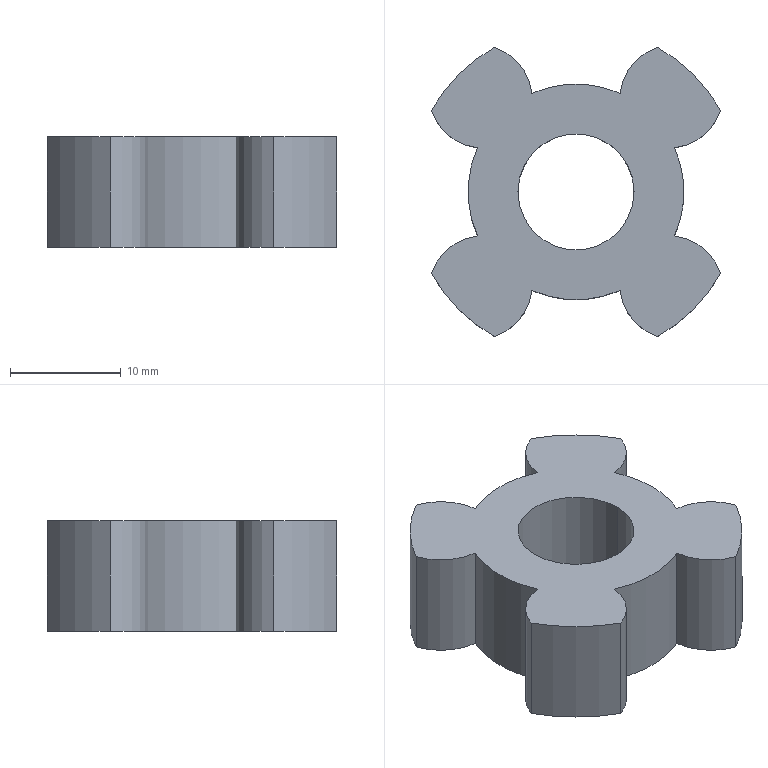Part | SolidWorks | features BaseBody 1 | 1 solid | 21 faces | box 26.134 x 26.134 x 10 mm | volume 3952 mm3 | cylinder 19 | plane 2 | commonest cylinder face diameters 10 x8 19.5 x5 30 x4 10.5 x2
STEP:
#1=CARTESIAN_POINT('',(5.25,0.,-5.));
#2=VERTEX_POINT('',#1);
#3=CARTESIAN_POINT('',(-5.25,0.,-5.));
#4=VERTEX_POINT('',#3);
#5=CARTESIAN_POINT('',(0.,0.,-5.));
#6=DIRECTION('',(0.,0.,-1.));
#7=DIRECTION('',(1.,0.,0.));
#8=AXIS2_PLACEMENT_3D('',#5,#6,#7);
#9=CIRCLE('',#8,5.25);
#10=EDGE_CURVE('',#2,#4,#9,.T.);
#11=ORIENTED_EDGE('',*,*,#10,.T.);
#12=CARTESIAN_POINT('',(-5.25,0.,5.));
#13=VERTEX_POINT('',#12);
#14=CARTESIAN_POINT('',(-5.25,0.,-5.));
#15=DIRECTION('',(0.,0.,1.));
#16=VECTOR('',#15,1000.);
#17=LINE('',#14,#16);
#18=EDGE_CURVE('',#4,#13,#17,.T.);
#19=ORIENTED_EDGE('',*,*,#18,.T.);
#20=CARTESIAN_POINT('',(5.25,0.,5.));
#21=VERTEX_POINT('',#20);
#22=CARTESIAN_POINT('',(0.,0.,5.));
#23=DIRECTION('',(0.,0.,-1.));
#24=DIRECTION('',(1.,0.,0.));
#25=AXIS2_PLACEMENT_3D('',#22,#23,#24);
#26=CIRCLE('',#25,5.25);
#27=EDGE_CURVE('',#21,#13,#26,.T.);
#28=ORIENTED_EDGE('',*,*,#27,.F.);
#29=CARTESIAN_POINT('',(5.25,0.,-5.));
#30=DIRECTION('',(0.,0.,1.));
#31=VECTOR('',#30,1000.);
#32=LINE('',#29,#31);
#33=EDGE_CURVE('',#2,#21,#32,.T.);
#34=ORIENTED_EDGE('',*,*,#33,.F.);
#35=EDGE_LOOP('',(#11,#19,#28,#34));
#36=FACE_OUTER_BOUND('',#35,.T.);
#37=CARTESIAN_POINT('',(0.,0.,-5.));
#38=DIRECTION('',(0.,0.,1.));
#39=DIRECTION('',(1.,0.,0.));
#40=AXIS2_PLACEMENT_3D('',#37,#38,#39);
#41=CYLINDRICAL_SURFACE('',#40,5.25);
#42=ADVANCED_FACE('',(#36),#41,.F.);
#43=CARTESIAN_POINT('',(8.901,-3.98,-5.));
#44=VERTEX_POINT('',#43);
#45=CARTESIAN_POINT('',(9.75,0.,-5.));
#46=VERTEX_POINT('',#45);
#47=CARTESIAN_POINT('',(0.,0.,-5.));
#48=DIRECTION('',(0.,0.,1.));
#49=DIRECTION('',(1.,0.,0.));
#50=AXIS2_PLACEMENT_3D('',#47,#48,#49);
#51=CIRCLE('',#50,9.75);
#52=EDGE_CURVE('',#44,#46,#51,.T.);
#53=ORIENTED_EDGE('',*,*,#52,.T.);
#54=CARTESIAN_POINT('',(9.75,0.,5.));
#55=VERTEX_POINT('',#54);
#56=CARTESIAN_POINT('',(9.75,0.,0.));
#57=DIRECTION('',(0.,0.,1.));
#58=VECTOR('',#57,1000.);
#59=LINE('',#56,#58);
#60=EDGE_CURVE('',#46,#55,#59,.T.);
#61=ORIENTED_EDGE('',*,*,#60,.T.);
#62=CARTESIAN_POINT('',(8.901,-3.98,5.));
#63=VERTEX_POINT('',#62);
#64=CARTESIAN_POINT('',(0.,0.,5.));
#65=DIRECTION('',(0.,0.,-1.));
#66=DIRECTION('',(1.,0.,0.));
#67=AXIS2_PLACEMENT_3D('',#64,#65,#66);
#68=CIRCLE('',#67,9.75);
#69=EDGE_CURVE('',#55,#63,#68,.T.);
#70=ORIENTED_EDGE('',*,*,#69,.T.);
#71=CARTESIAN_POINT('',(8.901,-3.98,0.));
#72=DIRECTION('',(0.,0.,-1.));
#73=VECTOR('',#72,1000.);
#74=LINE('',#71,#73);
#75=EDGE_CURVE('',#63,#44,#74,.T.);
#76=ORIENTED_EDGE('',*,*,#75,.T.);
#77=EDGE_LOOP('',(#53,#61,#70,#76));
#78=FACE_OUTER_BOUND('',#77,.T.);
#79=CARTESIAN_POINT('',(0.,0.,0.));
#80=DIRECTION('',(0.,0.,1.));
#81=DIRECTION('',(1.,0.,0.));
#82=AXIS2_PLACEMENT_3D('',#79,#80,#81);
#83=CYLINDRICAL_SURFACE('',#82,9.75);
#84=ADVANCED_FACE('',(#78),#83,.T.);
#85=ORIENTED_EDGE('',*,*,#10,.F.);
#86=CARTESIAN_POINT('',(0.,0.,-5.));
#87=DIRECTION('',(0.,0.,-1.));
#88=DIRECTION('',(1.,0.,0.));
#89=AXIS2_PLACEMENT_3D('',#86,#87,#88);
#90=CIRCLE('',#89,5.25);
#91=EDGE_CURVE('',#4,#2,#90,.T.);
#92=ORIENTED_EDGE('',*,*,#91,.F.);
#93=EDGE_LOOP('',(#85,#92));
#94=FACE_BOUND('',#93,.T.);
#95=CARTESIAN_POINT('',(7.366,13.067,-5.));
#96=VERTEX_POINT('',#95);
#97=CARTESIAN_POINT('',(3.98,8.901,-5.));
#98=VERTEX_POINT('',#97);
#99=CARTESIAN_POINT('',(8.946,8.323,-5.));
#100=DIRECTION('',(0.,0.,1.));
#101=DIRECTION('',(1.,0.,0.));
#102=AXIS2_PLACEMENT_3D('',#99,#100,#101);
#103=CIRCLE('',#102,5.);
#104=EDGE_CURVE('',#96,#98,#103,.T.);
#105=ORIENTED_EDGE('',*,*,#104,.F.);
#106=CARTESIAN_POINT('',(13.067,7.366,-5.));
#107=VERTEX_POINT('',#106);
#108=CARTESIAN_POINT('',(0.,0.,-5.));
#109=DIRECTION('',(0.,0.,1.));
#110=DIRECTION('',(1.,0.,0.));
#111=AXIS2_PLACEMENT_3D('',#108,#109,#110);
#112=CIRCLE('',#111,15.);
#113=EDGE_CURVE('',#107,#96,#112,.T.);
#114=ORIENTED_EDGE('',*,*,#113,.F.);
#115=CARTESIAN_POINT('',(8.901,3.98,-5.));
#116=VERTEX_POINT('',#115);
#117=CARTESIAN_POINT('',(8.323,8.946,-5.));
#118=DIRECTION('',(0.,0.,1.));
#119=DIRECTION('',(1.,0.,0.));
#120=AXIS2_PLACEMENT_3D('',#117,#118,#119);
#121=CIRCLE('',#120,5.);
#122=EDGE_CURVE('',#116,#107,#121,.T.);
#123=ORIENTED_EDGE('',*,*,#122,.F.);
#124=CARTESIAN_POINT('',(0.,0.,-5.));
#125=DIRECTION('',(0.,0.,1.));
#126=DIRECTION('',(1.,0.,0.));
#127=AXIS2_PLACEMENT_3D('',#124,#125,#126);
#128=CIRCLE('',#127,9.75);
#129=EDGE_CURVE('',#46,#116,#128,.T.);
#130=ORIENTED_EDGE('',*,*,#129,.F.);
#131=ORIENTED_EDGE('',*,*,#52,.F.);
#132=CARTESIAN_POINT('',(13.067,-7.366,-5.));
#133=VERTEX_POINT('',#132);
#134=CARTESIAN_POINT('',(8.323,-8.946,-5.));
#135=DIRECTION('',(0.,0.,1.));
#136=DIRECTION('',(1.,0.,0.));
#137=AXIS2_PLACEMENT_3D('',#134,#135,#136);
#138=CIRCLE('',#137,5.);
#139=EDGE_CURVE('',#133,#44,#138,.T.);
#140=ORIENTED_EDGE('',*,*,#139,.F.);
#141=CARTESIAN_POINT('',(7.366,-13.067,-5.));
#142=VERTEX_POINT('',#141);
#143=CARTESIAN_POINT('',(0.,0.,-5.));
#144=DIRECTION('',(0.,0.,1.));
#145=DIRECTION('',(1.,0.,0.));
#146=AXIS2_PLACEMENT_3D('',#143,#144,#145);
#147=CIRCLE('',#146,15.);
#148=EDGE_CURVE('',#142,#133,#147,.T.);
#149=ORIENTED_EDGE('',*,*,#148,.F.);
#150=CARTESIAN_POINT('',(3.98,-8.901,-5.));
#151=VERTEX_POINT('',#150);
#152=CARTESIAN_POINT('',(8.946,-8.323,-5.));
#153=DIRECTION('',(0.,0.,1.));
#154=DIRECTION('',(1.,0.,0.));
#155=AXIS2_PLACEMENT_3D('',#152,#153,#154);
#156=CIRCLE('',#155,5.);
#157=EDGE_CURVE('',#151,#142,#156,.T.);
#158=ORIENTED_EDGE('',*,*,#157,.F.);
#159=CARTESIAN_POINT('',(-3.98,-8.901,-5.));
#160=VERTEX_POINT('',#159);
#161=CARTESIAN_POINT('',(0.,0.,-5.));
#162=DIRECTION('',(0.,0.,1.));
#163=DIRECTION('',(1.,0.,0.));
#164=AXIS2_PLACEMENT_3D('',#161,#162,#163);
#165=CIRCLE('',#164,9.75);
#166=EDGE_CURVE('',#160,#151,#165,.T.);
#167=ORIENTED_EDGE('',*,*,#166,.F.);
#168=CARTESIAN_POINT('',(-7.366,-13.067,-5.));
#169=VERTEX_POINT('',#168);
#170=CARTESIAN_POINT('',(-8.946,-8.323,-5.));
#171=DIRECTION('',(0.,0.,1.));
#172=DIRECTION('',(1.,0.,0.));
#173=AXIS2_PLACEMENT_3D('',#170,#171,#172);
#174=CIRCLE('',#173,5.);
#175=EDGE_CURVE('',#169,#160,#174,.T.);
#176=ORIENTED_EDGE('',*,*,#175,.F.);
#177=CARTESIAN_POINT('',(-13.067,-7.366,-5.));
#178=VERTEX_POINT('',#177);
#179=CARTESIAN_POINT('',(0.,0.,-5.));
#180=DIRECTION('',(0.,0.,1.));
#181=DIRECTION('',(1.,0.,0.));
#182=AXIS2_PLACEMENT_3D('',#179,#180,#181);
#183=CIRCLE('',#182,15.);
#184=EDGE_CURVE('',#178,#169,#183,.T.);
#185=ORIENTED_EDGE('',*,*,#184,.F.);
#186=CARTESIAN_POINT('',(-8.901,-3.98,-5.));
#187=VERTEX_POINT('',#186);
#188=CARTESIAN_POINT('',(-8.323,-8.946,-5.));
#189=DIRECTION('',(0.,0.,1.));
#190=DIRECTION('',(1.,0.,0.));
#191=AXIS2_PLACEMENT_3D('',#188,#189,#190);
#192=CIRCLE('',#191,5.);
#193=EDGE_CURVE('',#187,#178,#192,.T.);
#194=ORIENTED_EDGE('',*,*,#193,.F.);
#195=CARTESIAN_POINT('',(-8.901,3.98,-5.));
#196=VERTEX_POINT('',#195);
#197=CARTESIAN_POINT('',(0.,0.,-5.));
#198=DIRECTION('',(0.,0.,1.));
#199=DIRECTION('',(1.,0.,0.));
#200=AXIS2_PLACEMENT_3D('',#197,#198,#199);
#201=CIRCLE('',#200,9.75);
#202=EDGE_CURVE('',#196,#187,#201,.T.);
#203=ORIENTED_EDGE('',*,*,#202,.F.);
#204=CARTESIAN_POINT('',(-13.067,7.366,-5.));
#205=VERTEX_POINT('',#204);
#206=CARTESIAN_POINT('',(-8.323,8.946,-5.));
#207=DIRECTION('',(0.,0.,1.));
#208=DIRECTION('',(1.,0.,0.));
#209=AXIS2_PLACEMENT_3D('',#206,#207,#208);
#210=CIRCLE('',#209,5.);
#211=EDGE_CURVE('',#205,#196,#210,.T.);
#212=ORIENTED_EDGE('',*,*,#211,.F.);
#213=CARTESIAN_POINT('',(-7.366,13.067,-5.));
#214=VERTEX_POINT('',#213);
#215=CARTESIAN_POINT('',(0.,0.,-5.));
#216=DIRECTION('',(0.,0.,1.));
#217=DIRECTION('',(1.,0.,0.));
#218=AXIS2_PLACEMENT_3D('',#215,#216,#217);
#219=CIRCLE('',#218,15.);
#220=EDGE_CURVE('',#214,#205,#219,.T.);
#221=ORIENTED_EDGE('',*,*,#220,.F.);
#222=CARTESIAN_POINT('',(-3.98,8.901,-5.));
#223=VERTEX_POINT('',#222);
#224=CARTESIAN_POINT('',(-8.946,8.323,-5.));
#225=DIRECTION('',(0.,0.,1.));
#226=DIRECTION('',(1.,0.,0.));
#227=AXIS2_PLACEMENT_3D('',#224,#225,#226);
#228=CIRCLE('',#227,5.);
#229=EDGE_CURVE('',#223,#214,#228,.T.);
#230=ORIENTED_EDGE('',*,*,#229,.F.);
#231=CARTESIAN_POINT('',(0.,0.,-5.));
#232=DIRECTION('',(0.,0.,1.));
#233=DIRECTION('',(1.,0.,0.));
#234=AXIS2_PLACEMENT_3D('',#231,#232,#233);
#235=CIRCLE('',#234,9.75);
#236=EDGE_CURVE('',#98,#223,#235,.T.);
#237=ORIENTED_EDGE('',*,*,#236,.F.);
#238=EDGE_LOOP('',(#105,#114,#123,#130,#131,#140,#149,#158,#167,#176,#185,#194,#203,#212,#221,#230,#237));
#239=FACE_OUTER_BOUND('',#238,.T.);
#240=CARTESIAN_POINT('',(0.,0.,-5.));
#241=DIRECTION('',(0.,0.,1.));
#242=DIRECTION('',(1.,0.,0.));
#243=AXIS2_PLACEMENT_3D('',#240,#241,#242);
#244=PLANE('',#243);
#245=ADVANCED_FACE('',(#94,#239),#244,.F.);
#246=ORIENTED_EDGE('',*,*,#18,.F.);
#247=ORIENTED_EDGE('',*,*,#91,.T.);
#248=ORIENTED_EDGE('',*,*,#33,.T.);
#249=CARTESIAN_POINT('',(0.,0.,5.));
#250=DIRECTION('',(0.,0.,-1.));
#251=DIRECTION('',(1.,0.,0.));
#252=AXIS2_PLACEMENT_3D('',#249,#250,#251);
#253=CIRCLE('',#252,5.25);
#254=EDGE_CURVE('',#13,#21,#253,.T.);
#255=ORIENTED_EDGE('',*,*,#254,.F.);
#256=EDGE_LOOP('',(#246,#247,#248,#255));
#257=FACE_OUTER_BOUND('',#256,.T.);
#258=CARTESIAN_POINT('',(0.,0.,-5.));
#259=DIRECTION('',(0.,0.,1.));
#260=DIRECTION('',(1.,0.,0.));
#261=AXIS2_PLACEMENT_3D('',#258,#259,#260);
#262=CYLINDRICAL_SURFACE('',#261,5.25);
#263=ADVANCED_FACE('',(#257),#262,.F.);
#264=CARTESIAN_POINT('',(-3.98,8.901,5.));
#265=VERTEX_POINT('',#264);
#266=CARTESIAN_POINT('',(3.98,8.901,5.));
#267=VERTEX_POINT('',#266);
#268=CARTESIAN_POINT('',(0.,0.,5.));
#269=DIRECTION('',(0.,0.,-1.));
#270=DIRECTION('',(1.,0.,0.));
#271=AXIS2_PLACEMENT_3D('',#268,#269,#270);
#272=CIRCLE('',#271,9.75);
#273=EDGE_CURVE('',#265,#267,#272,.T.);
#274=ORIENTED_EDGE('',*,*,#273,.T.);
#275=CARTESIAN_POINT('',(3.98,8.901,0.));
#276=DIRECTION('',(0.,0.,-1.));
#277=VECTOR('',#276,1000.);
#278=LINE('',#275,#277);
#279=EDGE_CURVE('',#267,#98,#278,.T.);
#280=ORIENTED_EDGE('',*,*,#279,.T.);
#281=ORIENTED_EDGE('',*,*,#236,.T.);
#282=CARTESIAN_POINT('',(-3.98,8.901,0.));
#283=DIRECTION('',(0.,0.,1.));
#284=VECTOR('',#283,1000.);
#285=LINE('',#282,#284);
#286=EDGE_CURVE('',#223,#265,#285,.T.);
#287=ORIENTED_EDGE('',*,*,#286,.T.);
#288=EDGE_LOOP('',(#274,#280,#281,#287));
#289=FACE_OUTER_BOUND('',#288,.T.);
#290=CARTESIAN_POINT('',(0.,0.,0.));
#291=DIRECTION('',(0.,0.,1.));
#292=DIRECTION('',(1.,0.,0.));
#293=AXIS2_PLACEMENT_3D('',#290,#291,#292);
#294=CYLINDRICAL_SURFACE('',#293,9.75);
#295=ADVANCED_FACE('',(#289),#294,.T.);
#296=CARTESIAN_POINT('',(7.366,13.067,5.));
#297=VERTEX_POINT('',#296);
#298=CARTESIAN_POINT('',(8.946,8.323,5.));
#299=DIRECTION('',(0.,0.,-1.));
#300=DIRECTION('',(1.,0.,0.));
#301=AXIS2_PLACEMENT_3D('',#298,#299,#300);
#302=CIRCLE('',#301,5.);
#303=EDGE_CURVE('',#267,#297,#302,.T.);
#304=ORIENTED_EDGE('',*,*,#303,.T.);
#305=CARTESIAN_POINT('',(7.366,13.067,0.));
#306=DIRECTION('',(0.,0.,-1.));
#307=VECTOR('',#306,1000.);
#308=LINE('',#305,#307);
#309=EDGE_CURVE('',#297,#96,#308,.T.);
#310=ORIENTED_EDGE('',*,*,#309,.T.);
#311=ORIENTED_EDGE('',*,*,#104,.T.);
#312=ORIENTED_EDGE('',*,*,#279,.F.);
#313=EDGE_LOOP('',(#304,#310,#311,#312));
#314=FACE_OUTER_BOUND('',#313,.T.);
#315=CARTESIAN_POINT('',(8.946,8.323,0.));
#316=DIRECTION('',(0.,0.,1.));
#317=DIRECTION('',(1.,0.,0.));
#318=AXIS2_PLACEMENT_3D('',#315,#316,#317);
#319=CYLINDRICAL_SURFACE('',#318,5.);
#320=ADVANCED_FACE('',(#314),#319,.T.);
#321=CARTESIAN_POINT('',(13.067,7.366,5.));
#322=VERTEX_POINT('',#321);
#323=CARTESIAN_POINT('',(0.,0.,5.));
#324=DIRECTION('',(0.,0.,-1.));
#325=DIRECTION('',(1.,0.,0.));
#326=AXIS2_PLACEMENT_3D('',#323,#324,#325);
#327=CIRCLE('',#326,15.);
#328=EDGE_CURVE('',#297,#322,#327,.T.);
#329=ORIENTED_EDGE('',*,*,#328,.T.);
#330=CARTESIAN_POINT('',(13.067,7.366,0.));
#331=DIRECTION('',(0.,0.,-1.));
#332=VECTOR('',#331,1000.);
#333=LINE('',#330,#332);
#334=EDGE_CURVE('',#322,#107,#333,.T.);
#335=ORIENTED_EDGE('',*,*,#334,.T.);
#336=ORIENTED_EDGE('',*,*,#113,.T.);
#337=ORIENTED_EDGE('',*,*,#309,.F.);
#338=EDGE_LOOP('',(#329,#335,#336,#337));
#339=FACE_OUTER_BOUND('',#338,.T.);
#340=CARTESIAN_POINT('',(0.,0.,0.));
#341=DIRECTION('',(0.,0.,1.));
#342=DIRECTION('',(1.,0.,0.));
#343=AXIS2_PLACEMENT_3D('',#340,#341,#342);
#344=CYLINDRICAL_SURFACE('',#343,15.);
#345=ADVANCED_FACE('',(#339),#344,.T.);
#346=CARTESIAN_POINT('',(8.901,3.98,5.));
#347=VERTEX_POINT('',#346);
#348=CARTESIAN_POINT('',(8.323,8.946,5.));
#349=DIRECTION('',(0.,0.,-1.));
#350=DIRECTION('',(1.,0.,0.));
#351=AXIS2_PLACEMENT_3D('',#348,#349,#350);
#352=CIRCLE('',#351,5.);
#353=EDGE_CURVE('',#322,#347,#352,.T.);
#354=ORIENTED_EDGE('',*,*,#353,.T.);
#355=CARTESIAN_POINT('',(8.901,3.98,0.));
#356=DIRECTION('',(0.,0.,-1.));
#357=VECTOR('',#356,1000.);
#358=LINE('',#355,#357);
#359=EDGE_CURVE('',#347,#116,#358,.T.);
#360=ORIENTED_EDGE('',*,*,#359,.T.);
#361=ORIENTED_EDGE('',*,*,#122,.T.);
#362=ORIENTED_EDGE('',*,*,#334,.F.);
#363=EDGE_LOOP('',(#354,#360,#361,#362));
#364=FACE_OUTER_BOUND('',#363,.T.);
#365=CARTESIAN_POINT('',(8.323,8.946,0.));
#366=DIRECTION('',(0.,0.,1.));
#367=DIRECTION('',(1.,0.,0.));
#368=AXIS2_PLACEMENT_3D('',#365,#366,#367);
#369=CYLINDRICAL_SURFACE('',#368,5.);
#370=ADVANCED_FACE('',(#364),#369,.T.);
#371=ORIENTED_EDGE('',*,*,#60,.F.);
#372=ORIENTED_EDGE('',*,*,#129,.T.);
#373=ORIENTED_EDGE('',*,*,#359,.F.);
#374=CARTESIAN_POINT('',(0.,0.,5.));
#375=DIRECTION('',(0.,0.,-1.));
#376=DIRECTION('',(1.,0.,0.));
#377=AXIS2_PLACEMENT_3D('',#374,#375,#376);
#378=CIRCLE('',#377,9.75);
#379=EDGE_CURVE('',#347,#55,#378,.T.);
#380=ORIENTED_EDGE('',*,*,#379,.T.);
#381=EDGE_LOOP('',(#371,#372,#373,#380));
#382=FACE_OUTER_BOUND('',#381,.T.);
#383=CARTESIAN_POINT('',(0.,0.,0.));
#384=DIRECTION('',(0.,0.,1.));
#385=DIRECTION('',(1.,0.,0.));
#386=AXIS2_PLACEMENT_3D('',#383,#384,#385);
#387=CYLINDRICAL_SURFACE('',#386,9.75);
#388=ADVANCED_FACE('',(#382),#387,.T.);
#389=CARTESIAN_POINT('',(13.067,-7.366,5.));
#390=VERTEX_POINT('',#389);
#391=CARTESIAN_POINT('',(8.323,-8.946,5.));
#392=DIRECTION('',(0.,0.,-1.));
#393=DIRECTION('',(1.,0.,0.));
#394=AXIS2_PLACEMENT_3D('',#391,#392,#393);
#395=CIRCLE('',#394,5.);
#396=EDGE_CURVE('',#63,#390,#395,.T.);
#397=ORIENTED_EDGE('',*,*,#396,.T.);
#398=CARTESIAN_POINT('',(13.067,-7.366,0.));
#399=DIRECTION('',(0.,0.,-1.));
#400=VECTOR('',#399,1000.);
#401=LINE('',#398,#400);
#402=EDGE_CURVE('',#390,#133,#401,.T.);
#403=ORIENTED_EDGE('',*,*,#402,.T.);
#404=ORIENTED_EDGE('',*,*,#139,.T.);
#405=ORIENTED_EDGE('',*,*,#75,.F.);
#406=EDGE_LOOP('',(#397,#403,#404,#405));
#407=FACE_OUTER_BOUND('',#406,.T.);
#408=CARTESIAN_POINT('',(8.323,-8.946,0.));
#409=DIRECTION('',(0.,0.,1.));
#410=DIRECTION('',(1.,0.,0.));
#411=AXIS2_PLACEMENT_3D('',#408,#409,#410);
#412=CYLINDRICAL_SURFACE('',#411,5.);
#413=ADVANCED_FACE('',(#407),#412,.T.);
#414=CARTESIAN_POINT('',(7.366,-13.067,5.));
#415=VERTEX_POINT('',#414);
#416=CARTESIAN_POINT('',(0.,0.,5.));
#417=DIRECTION('',(0.,0.,-1.));
#418=DIRECTION('',(1.,0.,0.));
#419=AXIS2_PLACEMENT_3D('',#416,#417,#418);
#420=CIRCLE('',#419,15.);
#421=EDGE_CURVE('',#390,#415,#420,.T.);
#422=ORIENTED_EDGE('',*,*,#421,.T.);
#423=CARTESIAN_POINT('',(7.366,-13.067,0.));
#424=DIRECTION('',(0.,0.,-1.));
#425=VECTOR('',#424,1000.);
#426=LINE('',#423,#425);
#427=EDGE_CURVE('',#415,#142,#426,.T.);
#428=ORIENTED_EDGE('',*,*,#427,.T.);
#429=ORIENTED_EDGE('',*,*,#148,.T.);
#430=ORIENTED_EDGE('',*,*,#402,.F.);
#431=EDGE_LOOP('',(#422,#428,#429,#430));
#432=FACE_OUTER_BOUND('',#431,.T.);
#433=CARTESIAN_POINT('',(0.,0.,0.));
#434=DIRECTION('',(0.,0.,1.));
#435=DIRECTION('',(1.,0.,0.));
#436=AXIS2_PLACEMENT_3D('',#433,#434,#435);
#437=CYLINDRICAL_SURFACE('',#436,15.);
#438=ADVANCED_FACE('',(#432),#437,.T.);
#439=CARTESIAN_POINT('',(3.98,-8.901,5.));
#440=VERTEX_POINT('',#439);
#441=CARTESIAN_POINT('',(8.946,-8.323,5.));
#442=DIRECTION('',(0.,0.,-1.));
#443=DIRECTION('',(1.,0.,0.));
#444=AXIS2_PLACEMENT_3D('',#441,#442,#443);
#445=CIRCLE('',#444,5.);
#446=EDGE_CURVE('',#415,#440,#445,.T.);
#447=ORIENTED_EDGE('',*,*,#446,.T.);
#448=CARTESIAN_POINT('',(3.98,-8.901,0.));
#449=DIRECTION('',(0.,0.,-1.));
#450=VECTOR('',#449,1000.);
#451=LINE('',#448,#450);
#452=EDGE_CURVE('',#440,#151,#451,.T.);
#453=ORIENTED_EDGE('',*,*,#452,.T.);
#454=ORIENTED_EDGE('',*,*,#157,.T.);
#455=ORIENTED_EDGE('',*,*,#427,.F.);
#456=EDGE_LOOP('',(#447,#453,#454,#455));
#457=FACE_OUTER_BOUND('',#456,.T.);
#458=CARTESIAN_POINT('',(8.946,-8.323,0.));
#459=DIRECTION('',(0.,0.,1.));
#460=DIRECTION('',(1.,0.,0.));
#461=AXIS2_PLACEMENT_3D('',#458,#459,#460);
#462=CYLINDRICAL_SURFACE('',#461,5.);
#463=ADVANCED_FACE('',(#457),#462,.T.);
#464=CARTESIAN_POINT('',(-3.98,-8.901,5.));
#465=VERTEX_POINT('',#464);
#466=CARTESIAN_POINT('',(0.,0.,5.));
#467=DIRECTION('',(0.,0.,-1.));
#468=DIRECTION('',(1.,0.,0.));
#469=AXIS2_PLACEMENT_3D('',#466,#467,#468);
#470=CIRCLE('',#469,9.75);
#471=EDGE_CURVE('',#440,#465,#470,.T.);
#472=ORIENTED_EDGE('',*,*,#471,.T.);
#473=CARTESIAN_POINT('',(-3.98,-8.901,0.));
#474=DIRECTION('',(0.,0.,-1.));
#475=VECTOR('',#474,1000.);
#476=LINE('',#473,#475);
#477=EDGE_CURVE('',#465,#160,#476,.T.);
#478=ORIENTED_EDGE('',*,*,#477,.T.);
#479=ORIENTED_EDGE('',*,*,#166,.T.);
#480=ORIENTED_EDGE('',*,*,#452,.F.);
#481=EDGE_LOOP('',(#472,#478,#479,#480));
#482=FACE_OUTER_BOUND('',#481,.T.);
#483=CARTESIAN_POINT('',(0.,0.,0.));
#484=DIRECTION('',(0.,0.,1.));
#485=DIRECTION('',(1.,0.,0.));
#486=AXIS2_PLACEMENT_3D('',#483,#484,#485);
#487=CYLINDRICAL_SURFACE('',#486,9.75);
#488=ADVANCED_FACE('',(#482),#487,.T.);
#489=CARTESIAN_POINT('',(-7.366,-13.067,5.));
#490=VERTEX_POINT('',#489);
#491=CARTESIAN_POINT('',(-8.946,-8.323,5.));
#492=DIRECTION('',(0.,0.,-1.));
#493=DIRECTION('',(1.,0.,0.));
#494=AXIS2_PLACEMENT_3D('',#491,#492,#493);
#495=CIRCLE('',#494,5.);
#496=EDGE_CURVE('',#465,#490,#495,.T.);
#497=ORIENTED_EDGE('',*,*,#496,.T.);
#498=CARTESIAN_POINT('',(-7.366,-13.067,0.));
#499=DIRECTION('',(0.,0.,-1.));
#500=VECTOR('',#499,1000.);
#501=LINE('',#498,#500);
#502=EDGE_CURVE('',#490,#169,#501,.T.);
#503=ORIENTED_EDGE('',*,*,#502,.T.);
#504=ORIENTED_EDGE('',*,*,#175,.T.);
#505=ORIENTED_EDGE('',*,*,#477,.F.);
#506=EDGE_LOOP('',(#497,#503,#504,#505));
#507=FACE_OUTER_BOUND('',#506,.T.);
#508=CARTESIAN_POINT('',(-8.946,-8.323,0.));
#509=DIRECTION('',(0.,0.,1.));
#510=DIRECTION('',(1.,0.,0.));
#511=AXIS2_PLACEMENT_3D('',#508,#509,#510);
#512=CYLINDRICAL_SURFACE('',#511,5.);
#513=ADVANCED_FACE('',(#507),#512,.T.);
#514=CARTESIAN_POINT('',(-13.067,-7.366,5.));
#515=VERTEX_POINT('',#514);
#516=CARTESIAN_POINT('',(0.,0.,5.));
#517=DIRECTION('',(0.,0.,-1.));
#518=DIRECTION('',(1.,0.,0.));
#519=AXIS2_PLACEMENT_3D('',#516,#517,#518);
#520=CIRCLE('',#519,15.);
#521=EDGE_CURVE('',#490,#515,#520,.T.);
#522=ORIENTED_EDGE('',*,*,#521,.T.);
#523=CARTESIAN_POINT('',(-13.067,-7.366,0.));
#524=DIRECTION('',(0.,0.,-1.));
#525=VECTOR('',#524,1000.);
#526=LINE('',#523,#525);
#527=EDGE_CURVE('',#515,#178,#526,.T.);
#528=ORIENTED_EDGE('',*,*,#527,.T.);
#529=ORIENTED_EDGE('',*,*,#184,.T.);
#530=ORIENTED_EDGE('',*,*,#502,.F.);
#531=EDGE_LOOP('',(#522,#528,#529,#530));
#532=FACE_OUTER_BOUND('',#531,.T.);
#533=CARTESIAN_POINT('',(0.,0.,0.));
#534=DIRECTION('',(0.,0.,1.));
#535=DIRECTION('',(1.,0.,0.));
#536=AXIS2_PLACEMENT_3D('',#533,#534,#535);
#537=CYLINDRICAL_SURFACE('',#536,15.);
#538=ADVANCED_FACE('',(#532),#537,.T.);
#539=CARTESIAN_POINT('',(-8.901,-3.98,5.));
#540=VERTEX_POINT('',#539);
#541=CARTESIAN_POINT('',(-8.323,-8.946,5.));
#542=DIRECTION('',(0.,0.,-1.));
#543=DIRECTION('',(1.,0.,0.));
#544=AXIS2_PLACEMENT_3D('',#541,#542,#543);
#545=CIRCLE('',#544,5.);
#546=EDGE_CURVE('',#515,#540,#545,.T.);
#547=ORIENTED_EDGE('',*,*,#546,.T.);
#548=CARTESIAN_POINT('',(-8.901,-3.98,0.));
#549=DIRECTION('',(0.,0.,-1.));
#550=VECTOR('',#549,1000.);
#551=LINE('',#548,#550);
#552=EDGE_CURVE('',#540,#187,#551,.T.);
#553=ORIENTED_EDGE('',*,*,#552,.T.);
#554=ORIENTED_EDGE('',*,*,#193,.T.);
#555=ORIENTED_EDGE('',*,*,#527,.F.);
#556=EDGE_LOOP('',(#547,#553,#554,#555));
#557=FACE_OUTER_BOUND('',#556,.T.);
#558=CARTESIAN_POINT('',(-8.323,-8.946,0.));
#559=DIRECTION('',(0.,0.,1.));
#560=DIRECTION('',(1.,0.,0.));
#561=AXIS2_PLACEMENT_3D('',#558,#559,#560);
#562=CYLINDRICAL_SURFACE('',#561,5.);
#563=ADVANCED_FACE('',(#557),#562,.T.);
#564=CARTESIAN_POINT('',(-8.901,3.98,5.));
#565=VERTEX_POINT('',#564);
#566=CARTESIAN_POINT('',(0.,0.,5.));
#567=DIRECTION('',(0.,0.,-1.));
#568=DIRECTION('',(1.,0.,0.));
#569=AXIS2_PLACEMENT_3D('',#566,#567,#568);
#570=CIRCLE('',#569,9.75);
#571=EDGE_CURVE('',#540,#565,#570,.T.);
#572=ORIENTED_EDGE('',*,*,#571,.T.);
#573=CARTESIAN_POINT('',(-8.901,3.98,0.));
#574=DIRECTION('',(0.,0.,-1.));
#575=VECTOR('',#574,1000.);
#576=LINE('',#573,#575);
#577=EDGE_CURVE('',#565,#196,#576,.T.);
#578=ORIENTED_EDGE('',*,*,#577,.T.);
#579=ORIENTED_EDGE('',*,*,#202,.T.);
#580=ORIENTED_EDGE('',*,*,#552,.F.);
#581=EDGE_LOOP('',(#572,#578,#579,#580));
#582=FACE_OUTER_BOUND('',#581,.T.);
#583=CARTESIAN_POINT('',(0.,0.,0.));
#584=DIRECTION('',(0.,0.,1.));
#585=DIRECTION('',(1.,0.,0.));
#586=AXIS2_PLACEMENT_3D('',#583,#584,#585);
#587=CYLINDRICAL_SURFACE('',#586,9.75);
#588=ADVANCED_FACE('',(#582),#587,.T.);
#589=CARTESIAN_POINT('',(-13.067,7.366,5.));
#590=VERTEX_POINT('',#589);
#591=CARTESIAN_POINT('',(-8.323,8.946,5.));
#592=DIRECTION('',(0.,0.,-1.));
#593=DIRECTION('',(1.,0.,0.));
#594=AXIS2_PLACEMENT_3D('',#591,#592,#593);
#595=CIRCLE('',#594,5.);
#596=EDGE_CURVE('',#565,#590,#595,.T.);
#597=ORIENTED_EDGE('',*,*,#596,.T.);
#598=CARTESIAN_POINT('',(-13.067,7.366,0.));
#599=DIRECTION('',(0.,0.,-1.));
#600=VECTOR('',#599,1000.);
#601=LINE('',#598,#600);
#602=EDGE_CURVE('',#590,#205,#601,.T.);
#603=ORIENTED_EDGE('',*,*,#602,.T.);
#604=ORIENTED_EDGE('',*,*,#211,.T.);
#605=ORIENTED_EDGE('',*,*,#577,.F.);
#606=EDGE_LOOP('',(#597,#603,#604,#605));
#607=FACE_OUTER_BOUND('',#606,.T.);
#608=CARTESIAN_POINT('',(-8.323,8.946,0.));
#609=DIRECTION('',(0.,0.,1.));
#610=DIRECTION('',(1.,0.,0.));
#611=AXIS2_PLACEMENT_3D('',#608,#609,#610);
#612=CYLINDRICAL_SURFACE('',#611,5.);
#613=ADVANCED_FACE('',(#607),#612,.T.);
#614=CARTESIAN_POINT('',(-7.366,13.067,5.));
#615=VERTEX_POINT('',#614);
#616=CARTESIAN_POINT('',(0.,0.,5.));
#617=DIRECTION('',(0.,0.,-1.));
#618=DIRECTION('',(1.,0.,0.));
#619=AXIS2_PLACEMENT_3D('',#616,#617,#618);
#620=CIRCLE('',#619,15.);
#621=EDGE_CURVE('',#590,#615,#620,.T.);
#622=ORIENTED_EDGE('',*,*,#621,.T.);
#623=CARTESIAN_POINT('',(-7.366,13.067,0.));
#624=DIRECTION('',(0.,0.,-1.));
#625=VECTOR('',#624,1000.);
#626=LINE('',#623,#625);
#627=EDGE_CURVE('',#615,#214,#626,.T.);
#628=ORIENTED_EDGE('',*,*,#627,.T.);
#629=ORIENTED_EDGE('',*,*,#220,.T.);
#630=ORIENTED_EDGE('',*,*,#602,.F.);
#631=EDGE_LOOP('',(#622,#628,#629,#630));
#632=FACE_OUTER_BOUND('',#631,.T.);
#633=CARTESIAN_POINT('',(0.,0.,0.));
#634=DIRECTION('',(0.,0.,1.));
#635=DIRECTION('',(1.,0.,0.));
#636=AXIS2_PLACEMENT_3D('',#633,#634,#635);
#637=CYLINDRICAL_SURFACE('',#636,15.);
#638=ADVANCED_FACE('',(#632),#637,.T.);
#639=CARTESIAN_POINT('',(-8.946,8.323,5.));
#640=DIRECTION('',(0.,0.,-1.));
#641=DIRECTION('',(1.,0.,0.));
#642=AXIS2_PLACEMENT_3D('',#639,#640,#641);
#643=CIRCLE('',#642,5.);
#644=EDGE_CURVE('',#615,#265,#643,.T.);
#645=ORIENTED_EDGE('',*,*,#644,.T.);
#646=ORIENTED_EDGE('',*,*,#286,.F.);
#647=ORIENTED_EDGE('',*,*,#229,.T.);
#648=ORIENTED_EDGE('',*,*,#627,.F.);
#649=EDGE_LOOP('',(#645,#646,#647,#648));
#650=FACE_OUTER_BOUND('',#649,.T.);
#651=CARTESIAN_POINT('',(-8.946,8.323,0.));
#652=DIRECTION('',(0.,0.,1.));
#653=DIRECTION('',(1.,0.,0.));
#654=AXIS2_PLACEMENT_3D('',#651,#652,#653);
#655=CYLINDRICAL_SURFACE('',#654,5.);
#656=ADVANCED_FACE('',(#650),#655,.T.);
#657=ORIENTED_EDGE('',*,*,#27,.T.);
#658=ORIENTED_EDGE('',*,*,#254,.T.);
#659=EDGE_LOOP('',(#657,#658));
#660=FACE_BOUND('',#659,.T.);
#661=ORIENTED_EDGE('',*,*,#396,.F.);
#662=ORIENTED_EDGE('',*,*,#69,.F.);
#663=ORIENTED_EDGE('',*,*,#379,.F.);
#664=ORIENTED_EDGE('',*,*,#353,.F.);
#665=ORIENTED_EDGE('',*,*,#328,.F.);
#666=ORIENTED_EDGE('',*,*,#303,.F.);
#667=ORIENTED_EDGE('',*,*,#273,.F.);
#668=ORIENTED_EDGE('',*,*,#644,.F.);
#669=ORIENTED_EDGE('',*,*,#621,.F.);
#670=ORIENTED_EDGE('',*,*,#596,.F.);
#671=ORIENTED_EDGE('',*,*,#571,.F.);
#672=ORIENTED_EDGE('',*,*,#546,.F.);
#673=ORIENTED_EDGE('',*,*,#521,.F.);
#674=ORIENTED_EDGE('',*,*,#496,.F.);
#675=ORIENTED_EDGE('',*,*,#471,.F.);
#676=ORIENTED_EDGE('',*,*,#446,.F.);
#677=ORIENTED_EDGE('',*,*,#421,.F.);
#678=EDGE_LOOP('',(#661,#662,#663,#664,#665,#666,#667,#668,#669,#670,#671,#672,#673,#674,#675,#676,#677));
#679=FACE_OUTER_BOUND('',#678,.T.);
#680=CARTESIAN_POINT('',(0.,0.,5.));
#681=DIRECTION('',(0.,0.,1.));
#682=DIRECTION('',(1.,0.,0.));
#683=AXIS2_PLACEMENT_3D('',#680,#681,#682);
#684=PLANE('',#683);
#685=ADVANCED_FACE('',(#660,#679),#684,.T.);
#686=CLOSED_SHELL('',(#42,#84,#245,#263,#295,#320,#345,#370,#388,#413,#438,#463,#488,#513,#538,#563,#588,#613,#638,#656,#685));
#687=MANIFOLD_SOLID_BREP('',#686);
#688=CARTESIAN_POINT('',(0.,0.,0.));
#689=DIRECTION('',(0.,0.,1.));
#690=DIRECTION('',(1.,0.,0.));
#691=AXIS2_PLACEMENT_3D('',#688,#689,#690);
#692=(LENGTH_UNIT()NAMED_UNIT(*)SI_UNIT(.MILLI.,.METRE.));
#693=UNCERTAINTY_MEASURE_WITH_UNIT(LENGTH_MEASURE(0.00001),#692,'','');
#694=(NAMED_UNIT(*)PLANE_ANGLE_UNIT()SI_UNIT($,.RADIAN.));
#695=(NAMED_UNIT(*)SI_UNIT($,.STERADIAN.)SOLID_ANGLE_UNIT());
#696=(GEOMETRIC_REPRESENTATION_CONTEXT(3)GLOBAL_UNCERTAINTY_ASSIGNED_CONTEXT((#693))GLOBAL_UNIT_ASSIGNED_CONTEXT((#692,#694,#695))REPRESENTATION_CONTEXT('',''));
#697=ADVANCED_BREP_SHAPE_REPRESENTATION('',(#687,#691),#696);